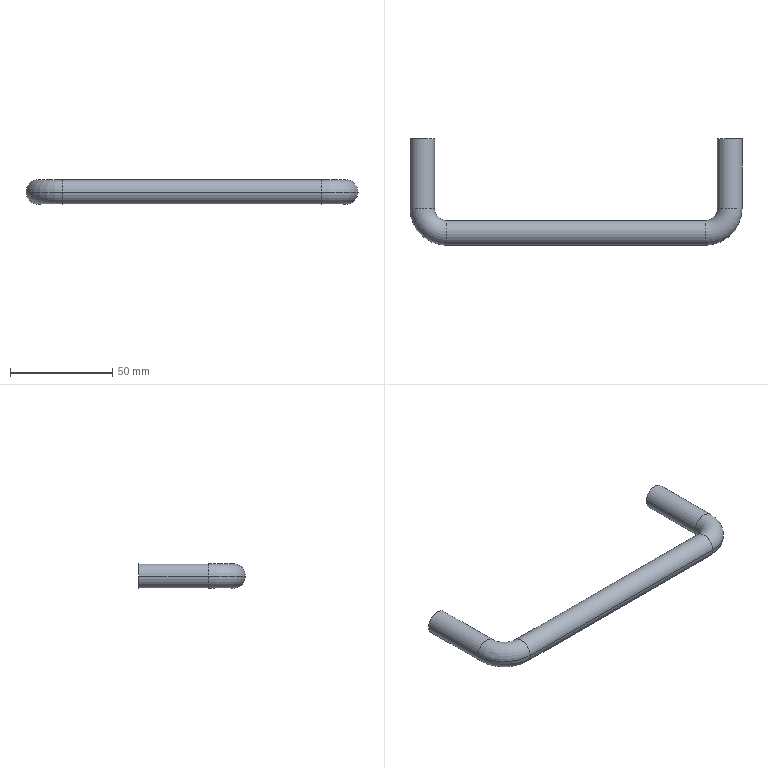Part | NX | 1 solid | 28 faces | box 162 x 52 x 12 mm | volume 24430 mm3 | cylinder 14 | cone 8 | torus 4 | plane 2 | commonest cylinder face diameters 6.8 x8 12 x6
STEP:
#1=CARTESIAN_POINT('',(-81.,0.,0.));
#2=VERTEX_POINT('',#1);
#3=CARTESIAN_POINT('',(-69.,0.,0.));
#4=VERTEX_POINT('',#3);
#5=CARTESIAN_POINT('',(-75.,0.,0.));
#6=DIRECTION('',(0.,-1.,0.));
#7=DIRECTION('',(1.,0.,0.));
#8=AXIS2_PLACEMENT_3D('',#5,#6,#7);
#9=CIRCLE('',#8,6.);
#10=EDGE_CURVE('',#2,#4,#9,.T.);
#11=ORIENTED_EDGE('',*,*,#10,.F.);
#12=CARTESIAN_POINT('',(-75.,0.,0.));
#13=DIRECTION('',(0.,-1.,0.));
#14=DIRECTION('',(1.,0.,0.));
#15=AXIS2_PLACEMENT_3D('',#12,#13,#14);
#16=CIRCLE('',#15,6.);
#17=EDGE_CURVE('',#4,#2,#16,.T.);
#18=ORIENTED_EDGE('',*,*,#17,.F.);
#19=EDGE_LOOP('',(#11,#18));
#20=FACE_BOUND('',#19,.T.);
#21=CARTESIAN_POINT('',(-79.562,0.,0.));
#22=VERTEX_POINT('',#21);
#23=CARTESIAN_POINT('',(-70.438,0.,0.));
#24=VERTEX_POINT('',#23);
#25=CARTESIAN_POINT('',(-75.,0.,0.));
#26=DIRECTION('',(0.,1.,0.));
#27=DIRECTION('',(1.,0.,0.));
#28=AXIS2_PLACEMENT_3D('',#25,#26,#27);
#29=CIRCLE('',#28,4.562);
#30=EDGE_CURVE('',#22,#24,#29,.T.);
#31=ORIENTED_EDGE('',*,*,#30,.F.);
#32=CARTESIAN_POINT('',(-75.,0.,0.));
#33=DIRECTION('',(0.,1.,0.));
#34=DIRECTION('',(1.,0.,0.));
#35=AXIS2_PLACEMENT_3D('',#32,#33,#34);
#36=CIRCLE('',#35,4.562);
#37=EDGE_CURVE('',#24,#22,#36,.T.);
#38=ORIENTED_EDGE('',*,*,#37,.F.);
#39=EDGE_LOOP('',(#31,#38));
#40=FACE_BOUND('',#39,.T.);
#41=CARTESIAN_POINT('',(-75.,0.,0.));
#42=DIRECTION('',(0.,-1.,0.));
#43=DIRECTION('',(0.,0.,-1.));
#44=AXIS2_PLACEMENT_3D('',#41,#42,#43);
#45=PLANE('',#44);
#46=ADVANCED_FACE('',(#20,#40),#45,.F.);
#47=CARTESIAN_POINT('',(-81.,-34.,0.));
#48=VERTEX_POINT('',#47);
#49=CARTESIAN_POINT('',(-69.,-34.,0.));
#50=VERTEX_POINT('',#49);
#51=CARTESIAN_POINT('',(-75.,-34.,0.));
#52=DIRECTION('',(0.,1.,0.));
#53=DIRECTION('',(1.,0.,0.));
#54=AXIS2_PLACEMENT_3D('',#51,#52,#53);
#55=CIRCLE('',#54,6.);
#56=EDGE_CURVE('',#48,#50,#55,.T.);
#57=ORIENTED_EDGE('',*,*,#56,.T.);
#58=CARTESIAN_POINT('',(-69.,0.,0.));
#59=DIRECTION('',(0.,-1.,0.));
#60=VECTOR('',#59,1000.);
#61=LINE('',#58,#60);
#62=EDGE_CURVE('',#4,#50,#61,.T.);
#63=ORIENTED_EDGE('',*,*,#62,.F.);
#64=ORIENTED_EDGE('',*,*,#17,.T.);
#65=CARTESIAN_POINT('',(-81.,0.,0.));
#66=DIRECTION('',(0.,-1.,0.));
#67=VECTOR('',#66,1000.);
#68=LINE('',#65,#67);
#69=EDGE_CURVE('',#2,#48,#68,.T.);
#70=ORIENTED_EDGE('',*,*,#69,.T.);
#71=EDGE_LOOP('',(#57,#63,#64,#70));
#72=FACE_BOUND('',#71,.T.);
#73=CARTESIAN_POINT('',(-75.,0.,0.));
#74=DIRECTION('',(0.,-1.,0.));
#75=DIRECTION('',(1.,0.,0.));
#76=AXIS2_PLACEMENT_3D('',#73,#74,#75);
#77=CYLINDRICAL_SURFACE('',#76,6.);
#78=ADVANCED_FACE('',(#72),#77,.T.);
#79=CARTESIAN_POINT('',(81.,0.,0.));
#80=VERTEX_POINT('',#79);
#81=CARTESIAN_POINT('',(69.,0.,0.));
#82=VERTEX_POINT('',#81);
#83=CARTESIAN_POINT('',(75.,0.,0.));
#84=DIRECTION('',(0.,1.,0.));
#85=DIRECTION('',(-1.,0.,0.));
#86=AXIS2_PLACEMENT_3D('',#83,#84,#85);
#87=CIRCLE('',#86,6.);
#88=EDGE_CURVE('',#80,#82,#87,.T.);
#89=ORIENTED_EDGE('',*,*,#88,.F.);
#90=CARTESIAN_POINT('',(81.,-34.,0.));
#91=VERTEX_POINT('',#90);
#92=CARTESIAN_POINT('',(81.,-34.,0.));
#93=DIRECTION('',(0.,1.,0.));
#94=VECTOR('',#93,1000.);
#95=LINE('',#92,#94);
#96=EDGE_CURVE('',#80,#91,#95,.F.);
#97=ORIENTED_EDGE('',*,*,#96,.T.);
#98=CARTESIAN_POINT('',(69.,-34.,0.));
#99=VERTEX_POINT('',#98);
#100=CARTESIAN_POINT('',(75.,-34.,0.));
#101=DIRECTION('',(0.,1.,0.));
#102=DIRECTION('',(1.,0.,0.));
#103=AXIS2_PLACEMENT_3D('',#100,#101,#102);
#104=CIRCLE('',#103,6.);
#105=EDGE_CURVE('',#91,#99,#104,.T.);
#106=ORIENTED_EDGE('',*,*,#105,.T.);
#107=CARTESIAN_POINT('',(69.,-34.,0.));
#108=DIRECTION('',(0.,1.,0.));
#109=VECTOR('',#108,1000.);
#110=LINE('',#107,#109);
#111=EDGE_CURVE('',#82,#99,#110,.F.);
#112=ORIENTED_EDGE('',*,*,#111,.F.);
#113=EDGE_LOOP('',(#89,#97,#106,#112));
#114=FACE_BOUND('',#113,.T.);
#115=CARTESIAN_POINT('',(75.,-34.,0.));
#116=DIRECTION('',(0.,1.,0.));
#117=DIRECTION('',(-1.,0.,0.));
#118=AXIS2_PLACEMENT_3D('',#115,#116,#117);
#119=CYLINDRICAL_SURFACE('',#118,6.);
#120=ADVANCED_FACE('',(#114),#119,.T.);
#121=ORIENTED_EDGE('',*,*,#56,.F.);
#122=CARTESIAN_POINT('',(-63.,-52.,0.));
#123=VERTEX_POINT('',#122);
#124=CARTESIAN_POINT('',(-63.,-34.,0.));
#125=DIRECTION('',(0.,0.,1.));
#126=DIRECTION('',(1.,0.,0.));
#127=AXIS2_PLACEMENT_3D('',#124,#125,#126);
#128=CIRCLE('',#127,18.);
#129=EDGE_CURVE('',#123,#48,#128,.F.);
#130=ORIENTED_EDGE('',*,*,#129,.F.);
#131=CARTESIAN_POINT('',(-63.,-40.,0.));
#132=VERTEX_POINT('',#131);
#133=CARTESIAN_POINT('',(-63.,-46.,0.));
#134=DIRECTION('',(1.,0.,0.));
#135=DIRECTION('',(0.,-1.,0.));
#136=AXIS2_PLACEMENT_3D('',#133,#134,#135);
#137=CIRCLE('',#136,6.);
#138=EDGE_CURVE('',#132,#123,#137,.T.);
#139=ORIENTED_EDGE('',*,*,#138,.F.);
#140=CARTESIAN_POINT('',(-63.,-34.,0.));
#141=DIRECTION('',(0.,0.,1.));
#142=DIRECTION('',(1.,0.,0.));
#143=AXIS2_PLACEMENT_3D('',#140,#141,#142);
#144=CIRCLE('',#143,6.);
#145=EDGE_CURVE('',#132,#50,#144,.F.);
#146=ORIENTED_EDGE('',*,*,#145,.T.);
#147=EDGE_LOOP('',(#121,#130,#139,#146));
#148=FACE_BOUND('',#147,.T.);
#149=CARTESIAN_POINT('',(-63.,-34.,0.));
#150=DIRECTION('',(0.,0.,1.));
#151=DIRECTION('',(1.,0.,0.));
#152=AXIS2_PLACEMENT_3D('',#149,#150,#151);
#153=TOROIDAL_SURFACE('',#152,12.,6.);
#154=ADVANCED_FACE('',(#148),#153,.T.);
#155=ORIENTED_EDGE('',*,*,#88,.T.);
#156=CARTESIAN_POINT('',(75.,0.,0.));
#157=DIRECTION('',(0.,1.,0.));
#158=DIRECTION('',(-1.,0.,0.));
#159=AXIS2_PLACEMENT_3D('',#156,#157,#158);
#160=CIRCLE('',#159,6.);
#161=EDGE_CURVE('',#82,#80,#160,.T.);
#162=ORIENTED_EDGE('',*,*,#161,.T.);
#163=EDGE_LOOP('',(#155,#162));
#164=FACE_BOUND('',#163,.T.);
#165=CARTESIAN_POINT('',(70.438,0.,0.));
#166=VERTEX_POINT('',#165);
#167=CARTESIAN_POINT('',(79.562,0.,0.));
#168=VERTEX_POINT('',#167);
#169=CARTESIAN_POINT('',(75.,0.,0.));
#170=DIRECTION('',(0.,1.,0.));
#171=DIRECTION('',(1.,0.,0.));
#172=AXIS2_PLACEMENT_3D('',#169,#170,#171);
#173=CIRCLE('',#172,4.562);
#174=EDGE_CURVE('',#166,#168,#173,.T.);
#175=ORIENTED_EDGE('',*,*,#174,.F.);
#176=CARTESIAN_POINT('',(75.,0.,0.));
#177=DIRECTION('',(0.,1.,0.));
#178=DIRECTION('',(1.,0.,0.));
#179=AXIS2_PLACEMENT_3D('',#176,#177,#178);
#180=CIRCLE('',#179,4.562);
#181=EDGE_CURVE('',#168,#166,#180,.T.);
#182=ORIENTED_EDGE('',*,*,#181,.F.);
#183=EDGE_LOOP('',(#175,#182));
#184=FACE_BOUND('',#183,.T.);
#185=CARTESIAN_POINT('',(75.,0.,0.));
#186=DIRECTION('',(0.,1.,0.));
#187=DIRECTION('',(1.,0.,0.));
#188=AXIS2_PLACEMENT_3D('',#185,#186,#187);
#189=PLANE('',#188);
#190=ADVANCED_FACE('',(#164,#184),#189,.T.);
#191=CARTESIAN_POINT('',(-63.,-46.,0.));
#192=DIRECTION('',(1.,0.,0.));
#193=DIRECTION('',(0.,-1.,0.));
#194=AXIS2_PLACEMENT_3D('',#191,#192,#193);
#195=CIRCLE('',#194,6.);
#196=EDGE_CURVE('',#123,#132,#195,.T.);
#197=ORIENTED_EDGE('',*,*,#196,.T.);
#198=CARTESIAN_POINT('',(63.,-40.,0.));
#199=VERTEX_POINT('',#198);
#200=CARTESIAN_POINT('',(-63.,-40.,0.));
#201=DIRECTION('',(1.,0.,0.));
#202=VECTOR('',#201,1000.);
#203=LINE('',#200,#202);
#204=EDGE_CURVE('',#132,#199,#203,.T.);
#205=ORIENTED_EDGE('',*,*,#204,.T.);
#206=CARTESIAN_POINT('',(63.,-52.,0.));
#207=VERTEX_POINT('',#206);
#208=CARTESIAN_POINT('',(63.,-46.,0.));
#209=DIRECTION('',(-1.,0.,0.));
#210=DIRECTION('',(0.,1.,0.));
#211=AXIS2_PLACEMENT_3D('',#208,#209,#210);
#212=CIRCLE('',#211,6.);
#213=EDGE_CURVE('',#199,#207,#212,.T.);
#214=ORIENTED_EDGE('',*,*,#213,.T.);
#215=CARTESIAN_POINT('',(-63.,-52.,0.));
#216=DIRECTION('',(1.,0.,0.));
#217=VECTOR('',#216,1000.);
#218=LINE('',#215,#217);
#219=EDGE_CURVE('',#123,#207,#218,.T.);
#220=ORIENTED_EDGE('',*,*,#219,.F.);
#221=EDGE_LOOP('',(#197,#205,#214,#220));
#222=FACE_BOUND('',#221,.T.);
#223=CARTESIAN_POINT('',(-63.,-46.,0.));
#224=DIRECTION('',(1.,0.,0.));
#225=DIRECTION('',(0.,1.,0.));
#226=AXIS2_PLACEMENT_3D('',#223,#224,#225);
#227=CYLINDRICAL_SURFACE('',#226,6.);
#228=ADVANCED_FACE('',(#222),#227,.T.);
#229=ORIENTED_EDGE('',*,*,#105,.F.);
#230=CARTESIAN_POINT('',(63.,-34.,0.));
#231=DIRECTION('',(0.,0.,1.));
#232=DIRECTION('',(1.,0.,0.));
#233=AXIS2_PLACEMENT_3D('',#230,#231,#232);
#234=CIRCLE('',#233,18.);
#235=EDGE_CURVE('',#91,#207,#234,.F.);
#236=ORIENTED_EDGE('',*,*,#235,.T.);
#237=ORIENTED_EDGE('',*,*,#213,.F.);
#238=CARTESIAN_POINT('',(63.,-34.,0.));
#239=DIRECTION('',(0.,0.,1.));
#240=DIRECTION('',(1.,0.,0.));
#241=AXIS2_PLACEMENT_3D('',#238,#239,#240);
#242=CIRCLE('',#241,6.);
#243=EDGE_CURVE('',#99,#199,#242,.F.);
#244=ORIENTED_EDGE('',*,*,#243,.F.);
#245=EDGE_LOOP('',(#229,#236,#237,#244));
#246=FACE_BOUND('',#245,.T.);
#247=CARTESIAN_POINT('',(63.,-34.,0.));
#248=DIRECTION('',(0.,0.,1.));
#249=DIRECTION('',(1.,0.,0.));
#250=AXIS2_PLACEMENT_3D('',#247,#248,#249);
#251=TOROIDAL_SURFACE('',#250,12.,6.);
#252=ADVANCED_FACE('',(#246),#251,.T.);
#253=CARTESIAN_POINT('',(71.6,-0.6712,0.));
#254=VERTEX_POINT('',#253);
#255=CARTESIAN_POINT('',(78.4,-0.6712,0.));
#256=VERTEX_POINT('',#255);
#257=CARTESIAN_POINT('',(75.,-0.6712,0.));
#258=DIRECTION('',(0.,1.,0.));
#259=DIRECTION('',(1.,0.,0.));
#260=AXIS2_PLACEMENT_3D('',#257,#258,#259);
#261=CIRCLE('',#260,3.4);
#262=EDGE_CURVE('',#254,#256,#261,.T.);
#263=ORIENTED_EDGE('',*,*,#262,.T.);
#264=CARTESIAN_POINT('',(78.4,-16.,0.));
#265=VERTEX_POINT('',#264);
#266=CARTESIAN_POINT('',(78.4,0.,0.));
#267=DIRECTION('',(0.,1.,0.));
#268=VECTOR('',#267,1000.);
#269=LINE('',#266,#268);
#270=EDGE_CURVE('',#265,#256,#269,.T.);
#271=ORIENTED_EDGE('',*,*,#270,.F.);
#272=CARTESIAN_POINT('',(71.6,-16.,0.));
#273=VERTEX_POINT('',#272);
#274=CARTESIAN_POINT('',(75.,-16.,0.));
#275=DIRECTION('',(0.,1.,0.));
#276=DIRECTION('',(1.,0.,0.));
#277=AXIS2_PLACEMENT_3D('',#274,#275,#276);
#278=CIRCLE('',#277,3.4);
#279=EDGE_CURVE('',#273,#265,#278,.T.);
#280=ORIENTED_EDGE('',*,*,#279,.F.);
#281=CARTESIAN_POINT('',(71.6,0.,0.));
#282=DIRECTION('',(0.,1.,0.));
#283=VECTOR('',#282,1000.);
#284=LINE('',#281,#283);
#285=EDGE_CURVE('',#273,#254,#284,.T.);
#286=ORIENTED_EDGE('',*,*,#285,.T.);
#287=EDGE_LOOP('',(#263,#271,#280,#286));
#288=FACE_BOUND('',#287,.T.);
#289=CARTESIAN_POINT('',(75.,0.,0.));
#290=DIRECTION('',(0.,1.,0.));
#291=DIRECTION('',(1.,0.,0.));
#292=AXIS2_PLACEMENT_3D('',#289,#290,#291);
#293=CYLINDRICAL_SURFACE('',#292,3.4);
#294=ADVANCED_FACE('',(#288),#293,.F.);
#295=ORIENTED_EDGE('',*,*,#279,.T.);
#296=CARTESIAN_POINT('',(78.4,-23.5,0.));
#297=VERTEX_POINT('',#296);
#298=CARTESIAN_POINT('',(78.4,0.,0.));
#299=DIRECTION('',(0.,1.,0.));
#300=VECTOR('',#299,1000.);
#301=LINE('',#298,#300);
#302=EDGE_CURVE('',#297,#265,#301,.T.);
#303=ORIENTED_EDGE('',*,*,#302,.F.);
#304=CARTESIAN_POINT('',(71.6,-23.5,0.));
#305=VERTEX_POINT('',#304);
#306=CARTESIAN_POINT('',(75.,-23.5,0.));
#307=DIRECTION('',(0.,1.,0.));
#308=DIRECTION('',(1.,0.,0.));
#309=AXIS2_PLACEMENT_3D('',#306,#307,#308);
#310=CIRCLE('',#309,3.4);
#311=EDGE_CURVE('',#305,#297,#310,.T.);
#312=ORIENTED_EDGE('',*,*,#311,.F.);
#313=CARTESIAN_POINT('',(71.6,0.,0.));
#314=DIRECTION('',(0.,1.,0.));
#315=VECTOR('',#314,1000.);
#316=LINE('',#313,#315);
#317=EDGE_CURVE('',#305,#273,#316,.T.);
#318=ORIENTED_EDGE('',*,*,#317,.T.);
#319=EDGE_LOOP('',(#295,#303,#312,#318));
#320=FACE_BOUND('',#319,.T.);
#321=CARTESIAN_POINT('',(75.,0.,0.));
#322=DIRECTION('',(0.,1.,0.));
#323=DIRECTION('',(1.,0.,0.));
#324=AXIS2_PLACEMENT_3D('',#321,#322,#323);
#325=CYLINDRICAL_SURFACE('',#324,3.4);
#326=ADVANCED_FACE('',(#320),#325,.F.);
#327=ORIENTED_EDGE('',*,*,#311,.T.);
#328=CARTESIAN_POINT('',(75.,-25.543,0.));
#329=VERTEX_POINT('',#328);
#330=CARTESIAN_POINT('',(78.4,-23.5,0.));
#331=DIRECTION('',(0.8572,0.515,0.));
#332=VECTOR('',#331,1000.);
#333=LINE('',#330,#332);
#334=EDGE_CURVE('',#297,#329,#333,.F.);
#335=ORIENTED_EDGE('',*,*,#334,.T.);
#336=CARTESIAN_POINT('',(71.6,-23.5,0.));
#337=DIRECTION('',(-0.8572,0.515,0.));
#338=VECTOR('',#337,1000.);
#339=LINE('',#336,#338);
#340=EDGE_CURVE('',#305,#329,#339,.F.);
#341=ORIENTED_EDGE('',*,*,#340,.F.);
#342=EDGE_LOOP('',(#327,#335,#341));
#343=FACE_BOUND('',#342,.T.);
#344=CARTESIAN_POINT('',(75.,-23.5,0.));
#345=DIRECTION('',(0.,1.,0.));
#346=DIRECTION('',(1.,0.,0.));
#347=AXIS2_PLACEMENT_3D('',#344,#345,#346);
#348=CONICAL_SURFACE('',#347,3.4,1.03);
#349=ADVANCED_FACE('',(#343),#348,.F.);
#350=ORIENTED_EDGE('',*,*,#262,.F.);
#351=CARTESIAN_POINT('',(71.6,-0.6712,0.));
#352=DIRECTION('',(-0.866,0.5,0.));
#353=VECTOR('',#352,1000.);
#354=LINE('',#351,#353);
#355=EDGE_CURVE('',#254,#166,#354,.T.);
#356=ORIENTED_EDGE('',*,*,#355,.T.);
#357=ORIENTED_EDGE('',*,*,#174,.T.);
#358=CARTESIAN_POINT('',(78.4,-0.6712,0.));
#359=DIRECTION('',(0.866,0.5,0.));
#360=VECTOR('',#359,1000.);
#361=LINE('',#358,#360);
#362=EDGE_CURVE('',#256,#168,#361,.T.);
#363=ORIENTED_EDGE('',*,*,#362,.F.);
#364=EDGE_LOOP('',(#350,#356,#357,#363));
#365=FACE_BOUND('',#364,.T.);
#366=CARTESIAN_POINT('',(75.,-0.6712,0.));
#367=DIRECTION('',(0.,1.,0.));
#368=DIRECTION('',(1.,0.,0.));
#369=AXIS2_PLACEMENT_3D('',#366,#367,#368);
#370=CONICAL_SURFACE('',#369,3.4,1.047);
#371=ADVANCED_FACE('',(#365),#370,.F.);
#372=CARTESIAN_POINT('',(-78.4,-0.6712,0.));
#373=VERTEX_POINT('',#372);
#374=CARTESIAN_POINT('',(-71.6,-0.6712,0.));
#375=VERTEX_POINT('',#374);
#376=CARTESIAN_POINT('',(-75.,-0.6712,0.));
#377=DIRECTION('',(0.,1.,0.));
#378=DIRECTION('',(1.,0.,0.));
#379=AXIS2_PLACEMENT_3D('',#376,#377,#378);
#380=CIRCLE('',#379,3.4);
#381=EDGE_CURVE('',#373,#375,#380,.T.);
#382=ORIENTED_EDGE('',*,*,#381,.T.);
#383=CARTESIAN_POINT('',(-71.6,-16.,0.));
#384=VERTEX_POINT('',#383);
#385=CARTESIAN_POINT('',(-71.6,0.,0.));
#386=DIRECTION('',(0.,1.,0.));
#387=VECTOR('',#386,1000.);
#388=LINE('',#385,#387);
#389=EDGE_CURVE('',#384,#375,#388,.T.);
#390=ORIENTED_EDGE('',*,*,#389,.F.);
#391=CARTESIAN_POINT('',(-78.4,-16.,0.));
#392=VERTEX_POINT('',#391);
#393=CARTESIAN_POINT('',(-75.,-16.,0.));
#394=DIRECTION('',(0.,1.,0.));
#395=DIRECTION('',(1.,0.,0.));
#396=AXIS2_PLACEMENT_3D('',#393,#394,#395);
#397=CIRCLE('',#396,3.4);
#398=EDGE_CURVE('',#392,#384,#397,.T.);
#399=ORIENTED_EDGE('',*,*,#398,.F.);
#400=CARTESIAN_POINT('',(-78.4,0.,0.));
#401=DIRECTION('',(0.,1.,0.));
#402=VECTOR('',#401,1000.);
#403=LINE('',#400,#402);
#404=EDGE_CURVE('',#392,#373,#403,.T.);
#405=ORIENTED_EDGE('',*,*,#404,.T.);
#406=EDGE_LOOP('',(#382,#390,#399,#405));
#407=FACE_BOUND('',#406,.T.);
#408=CARTESIAN_POINT('',(-75.,0.,0.));
#409=DIRECTION('',(0.,1.,0.));
#410=DIRECTION('',(1.,0.,0.));
#411=AXIS2_PLACEMENT_3D('',#408,#409,#410);
#412=CYLINDRICAL_SURFACE('',#411,3.4);
#413=ADVANCED_FACE('',(#407),#412,.F.);
#414=ORIENTED_EDGE('',*,*,#398,.T.);
#415=CARTESIAN_POINT('',(-71.6,-23.5,0.));
#416=VERTEX_POINT('',#415);
#417=CARTESIAN_POINT('',(-71.6,0.,0.));
#418=DIRECTION('',(0.,1.,0.));
#419=VECTOR('',#418,1000.);
#420=LINE('',#417,#419);
#421=EDGE_CURVE('',#416,#384,#420,.T.);
#422=ORIENTED_EDGE('',*,*,#421,.F.);
#423=CARTESIAN_POINT('',(-78.4,-23.5,0.));
#424=VERTEX_POINT('',#423);
#425=CARTESIAN_POINT('',(-75.,-23.5,0.));
#426=DIRECTION('',(0.,1.,0.));
#427=DIRECTION('',(1.,0.,0.));
#428=AXIS2_PLACEMENT_3D('',#425,#426,#427);
#429=CIRCLE('',#428,3.4);
#430=EDGE_CURVE('',#424,#416,#429,.T.);
#431=ORIENTED_EDGE('',*,*,#430,.F.);
#432=CARTESIAN_POINT('',(-78.4,0.,0.));
#433=DIRECTION('',(0.,1.,0.));
#434=VECTOR('',#433,1000.);
#435=LINE('',#432,#434);
#436=EDGE_CURVE('',#424,#392,#435,.T.);
#437=ORIENTED_EDGE('',*,*,#436,.T.);
#438=EDGE_LOOP('',(#414,#422,#431,#437));
#439=FACE_BOUND('',#438,.T.);
#440=CARTESIAN_POINT('',(-75.,0.,0.));
#441=DIRECTION('',(0.,1.,0.));
#442=DIRECTION('',(1.,0.,0.));
#443=AXIS2_PLACEMENT_3D('',#440,#441,#442);
#444=CYLINDRICAL_SURFACE('',#443,3.4);
#445=ADVANCED_FACE('',(#439),#444,.F.);
#446=ORIENTED_EDGE('',*,*,#430,.T.);
#447=CARTESIAN_POINT('',(-75.,-25.543,0.));
#448=VERTEX_POINT('',#447);
#449=CARTESIAN_POINT('',(-71.6,-23.5,0.));
#450=DIRECTION('',(0.8572,0.515,0.));
#451=VECTOR('',#450,1000.);
#452=LINE('',#449,#451);
#453=EDGE_CURVE('',#416,#448,#452,.F.);
#454=ORIENTED_EDGE('',*,*,#453,.T.);
#455=CARTESIAN_POINT('',(-78.4,-23.5,0.));
#456=DIRECTION('',(-0.8572,0.515,0.));
#457=VECTOR('',#456,1000.);
#458=LINE('',#455,#457);
#459=EDGE_CURVE('',#424,#448,#458,.F.);
#460=ORIENTED_EDGE('',*,*,#459,.F.);
#461=EDGE_LOOP('',(#446,#454,#460));
#462=FACE_BOUND('',#461,.T.);
#463=CARTESIAN_POINT('',(-75.,-23.5,0.));
#464=DIRECTION('',(0.,1.,0.));
#465=DIRECTION('',(1.,0.,0.));
#466=AXIS2_PLACEMENT_3D('',#463,#464,#465);
#467=CONICAL_SURFACE('',#466,3.4,1.03);
#468=ADVANCED_FACE('',(#462),#467,.F.);
#469=ORIENTED_EDGE('',*,*,#381,.F.);
#470=CARTESIAN_POINT('',(-78.4,-0.6712,0.));
#471=DIRECTION('',(-0.866,0.5,0.));
#472=VECTOR('',#471,1000.);
#473=LINE('',#470,#472);
#474=EDGE_CURVE('',#373,#22,#473,.T.);
#475=ORIENTED_EDGE('',*,*,#474,.T.);
#476=ORIENTED_EDGE('',*,*,#30,.T.);
#477=CARTESIAN_POINT('',(-71.6,-0.6712,0.));
#478=DIRECTION('',(0.866,0.5,0.));
#479=VECTOR('',#478,1000.);
#480=LINE('',#477,#479);
#481=EDGE_CURVE('',#375,#24,#480,.T.);
#482=ORIENTED_EDGE('',*,*,#481,.F.);
#483=EDGE_LOOP('',(#469,#475,#476,#482));
#484=FACE_BOUND('',#483,.T.);
#485=CARTESIAN_POINT('',(-75.,-0.6712,0.));
#486=DIRECTION('',(0.,1.,0.));
#487=DIRECTION('',(1.,0.,0.));
#488=AXIS2_PLACEMENT_3D('',#485,#486,#487);
#489=CONICAL_SURFACE('',#488,3.4,1.047);
#490=ADVANCED_FACE('',(#484),#489,.F.);
#491=ORIENTED_EDGE('',*,*,#340,.T.);
#492=ORIENTED_EDGE('',*,*,#334,.F.);
#493=CARTESIAN_POINT('',(75.,-23.5,0.));
#494=DIRECTION('',(0.,1.,0.));
#495=DIRECTION('',(1.,0.,0.));
#496=AXIS2_PLACEMENT_3D('',#493,#494,#495);
#497=CIRCLE('',#496,3.4);
#498=EDGE_CURVE('',#297,#305,#497,.T.);
#499=ORIENTED_EDGE('',*,*,#498,.T.);
#500=EDGE_LOOP('',(#491,#492,#499));
#501=FACE_BOUND('',#500,.T.);
#502=CARTESIAN_POINT('',(75.,-23.5,0.));
#503=DIRECTION('',(0.,1.,0.));
#504=DIRECTION('',(1.,0.,0.));
#505=AXIS2_PLACEMENT_3D('',#502,#503,#504);
#506=CONICAL_SURFACE('',#505,3.4,1.03);
#507=ADVANCED_FACE('',(#501),#506,.F.);
#508=ORIENTED_EDGE('',*,*,#362,.T.);
#509=ORIENTED_EDGE('',*,*,#181,.T.);
#510=ORIENTED_EDGE('',*,*,#355,.F.);
#511=CARTESIAN_POINT('',(75.,-0.6712,0.));
#512=DIRECTION('',(0.,1.,0.));
#513=DIRECTION('',(1.,0.,0.));
#514=AXIS2_PLACEMENT_3D('',#511,#512,#513);
#515=CIRCLE('',#514,3.4);
#516=EDGE_CURVE('',#256,#254,#515,.T.);
#517=ORIENTED_EDGE('',*,*,#516,.F.);
#518=EDGE_LOOP('',(#508,#509,#510,#517));
#519=FACE_BOUND('',#518,.T.);
#520=CARTESIAN_POINT('',(75.,-0.6712,0.));
#521=DIRECTION('',(0.,1.,0.));
#522=DIRECTION('',(1.,0.,0.));
#523=AXIS2_PLACEMENT_3D('',#520,#521,#522);
#524=CONICAL_SURFACE('',#523,3.4,1.047);
#525=ADVANCED_FACE('',(#519),#524,.F.);
#526=ORIENTED_EDGE('',*,*,#111,.T.);
#527=CARTESIAN_POINT('',(75.,-34.,0.));
#528=DIRECTION('',(0.,1.,0.));
#529=DIRECTION('',(1.,0.,0.));
#530=AXIS2_PLACEMENT_3D('',#527,#528,#529);
#531=CIRCLE('',#530,6.);
#532=EDGE_CURVE('',#99,#91,#531,.T.);
#533=ORIENTED_EDGE('',*,*,#532,.T.);
#534=ORIENTED_EDGE('',*,*,#96,.F.);
#535=ORIENTED_EDGE('',*,*,#161,.F.);
#536=EDGE_LOOP('',(#526,#533,#534,#535));
#537=FACE_BOUND('',#536,.T.);
#538=CARTESIAN_POINT('',(75.,-34.,0.));
#539=DIRECTION('',(0.,1.,0.));
#540=DIRECTION('',(-1.,0.,0.));
#541=AXIS2_PLACEMENT_3D('',#538,#539,#540);
#542=CYLINDRICAL_SURFACE('',#541,6.);
#543=ADVANCED_FACE('',(#537),#542,.T.);
#544=ORIENTED_EDGE('',*,*,#196,.F.);
#545=ORIENTED_EDGE('',*,*,#129,.T.);
#546=CARTESIAN_POINT('',(-75.,-34.,0.));
#547=DIRECTION('',(0.,1.,0.));
#548=DIRECTION('',(1.,0.,0.));
#549=AXIS2_PLACEMENT_3D('',#546,#547,#548);
#550=CIRCLE('',#549,6.);
#551=EDGE_CURVE('',#50,#48,#550,.T.);
#552=ORIENTED_EDGE('',*,*,#551,.F.);
#553=ORIENTED_EDGE('',*,*,#145,.F.);
#554=EDGE_LOOP('',(#544,#545,#552,#553));
#555=FACE_BOUND('',#554,.T.);
#556=CARTESIAN_POINT('',(-63.,-34.,0.));
#557=DIRECTION('',(0.,0.,1.));
#558=DIRECTION('',(1.,0.,0.));
#559=AXIS2_PLACEMENT_3D('',#556,#557,#558);
#560=TOROIDAL_SURFACE('',#559,12.,6.);
#561=ADVANCED_FACE('',(#555),#560,.T.);
#562=ORIENTED_EDGE('',*,*,#421,.T.);
#563=CARTESIAN_POINT('',(-75.,-16.,0.));
#564=DIRECTION('',(0.,1.,0.));
#565=DIRECTION('',(1.,0.,0.));
#566=AXIS2_PLACEMENT_3D('',#563,#564,#565);
#567=CIRCLE('',#566,3.4);
#568=EDGE_CURVE('',#384,#392,#567,.T.);
#569=ORIENTED_EDGE('',*,*,#568,.T.);
#570=ORIENTED_EDGE('',*,*,#436,.F.);
#571=CARTESIAN_POINT('',(-75.,-23.5,0.));
#572=DIRECTION('',(0.,1.,0.));
#573=DIRECTION('',(1.,0.,0.));
#574=AXIS2_PLACEMENT_3D('',#571,#572,#573);
#575=CIRCLE('',#574,3.4);
#576=EDGE_CURVE('',#416,#424,#575,.T.);
#577=ORIENTED_EDGE('',*,*,#576,.F.);
#578=EDGE_LOOP('',(#562,#569,#570,#577));
#579=FACE_BOUND('',#578,.T.);
#580=CARTESIAN_POINT('',(-75.,0.,0.));
#581=DIRECTION('',(0.,1.,0.));
#582=DIRECTION('',(1.,0.,0.));
#583=AXIS2_PLACEMENT_3D('',#580,#581,#582);
#584=CYLINDRICAL_SURFACE('',#583,3.4);
#585=ADVANCED_FACE('',(#579),#584,.F.);
#586=ORIENTED_EDGE('',*,*,#270,.T.);
#587=ORIENTED_EDGE('',*,*,#516,.T.);
#588=ORIENTED_EDGE('',*,*,#285,.F.);
#589=CARTESIAN_POINT('',(75.,-16.,0.));
#590=DIRECTION('',(0.,1.,0.));
#591=DIRECTION('',(1.,0.,0.));
#592=AXIS2_PLACEMENT_3D('',#589,#590,#591);
#593=CIRCLE('',#592,3.4);
#594=EDGE_CURVE('',#265,#273,#593,.T.);
#595=ORIENTED_EDGE('',*,*,#594,.F.);
#596=EDGE_LOOP('',(#586,#587,#588,#595));
#597=FACE_BOUND('',#596,.T.);
#598=CARTESIAN_POINT('',(75.,0.,0.));
#599=DIRECTION('',(0.,1.,0.));
#600=DIRECTION('',(1.,0.,0.));
#601=AXIS2_PLACEMENT_3D('',#598,#599,#600);
#602=CYLINDRICAL_SURFACE('',#601,3.4);
#603=ADVANCED_FACE('',(#597),#602,.F.);
#604=CARTESIAN_POINT('',(63.,-46.,0.));
#605=DIRECTION('',(-1.,0.,0.));
#606=DIRECTION('',(0.,1.,0.));
#607=AXIS2_PLACEMENT_3D('',#604,#605,#606);
#608=CIRCLE('',#607,6.);
#609=EDGE_CURVE('',#207,#199,#608,.T.);
#610=ORIENTED_EDGE('',*,*,#609,.T.);
#611=ORIENTED_EDGE('',*,*,#204,.F.);
#612=ORIENTED_EDGE('',*,*,#138,.T.);
#613=ORIENTED_EDGE('',*,*,#219,.T.);
#614=EDGE_LOOP('',(#610,#611,#612,#613));
#615=FACE_BOUND('',#614,.T.);
#616=CARTESIAN_POINT('',(-63.,-46.,0.));
#617=DIRECTION('',(1.,0.,0.));
#618=DIRECTION('',(0.,1.,0.));
#619=AXIS2_PLACEMENT_3D('',#616,#617,#618);
#620=CYLINDRICAL_SURFACE('',#619,6.);
#621=ADVANCED_FACE('',(#615),#620,.T.);
#622=ORIENTED_EDGE('',*,*,#459,.T.);
#623=ORIENTED_EDGE('',*,*,#453,.F.);
#624=ORIENTED_EDGE('',*,*,#576,.T.);
#625=EDGE_LOOP('',(#622,#623,#624));
#626=FACE_BOUND('',#625,.T.);
#627=CARTESIAN_POINT('',(-75.,-23.5,0.));
#628=DIRECTION('',(0.,1.,0.));
#629=DIRECTION('',(1.,0.,0.));
#630=AXIS2_PLACEMENT_3D('',#627,#628,#629);
#631=CONICAL_SURFACE('',#630,3.4,1.03);
#632=ADVANCED_FACE('',(#626),#631,.F.);
#633=ORIENTED_EDGE('',*,*,#481,.T.);
#634=ORIENTED_EDGE('',*,*,#37,.T.);
#635=ORIENTED_EDGE('',*,*,#474,.F.);
#636=CARTESIAN_POINT('',(-75.,-0.6712,0.));
#637=DIRECTION('',(0.,1.,0.));
#638=DIRECTION('',(1.,0.,0.));
#639=AXIS2_PLACEMENT_3D('',#636,#637,#638);
#640=CIRCLE('',#639,3.4);
#641=EDGE_CURVE('',#375,#373,#640,.T.);
#642=ORIENTED_EDGE('',*,*,#641,.F.);
#643=EDGE_LOOP('',(#633,#634,#635,#642));
#644=FACE_BOUND('',#643,.T.);
#645=CARTESIAN_POINT('',(-75.,-0.6712,0.));
#646=DIRECTION('',(0.,1.,0.));
#647=DIRECTION('',(1.,0.,0.));
#648=AXIS2_PLACEMENT_3D('',#645,#646,#647);
#649=CONICAL_SURFACE('',#648,3.4,1.047);
#650=ADVANCED_FACE('',(#644),#649,.F.);
#651=ORIENTED_EDGE('',*,*,#302,.T.);
#652=ORIENTED_EDGE('',*,*,#594,.T.);
#653=ORIENTED_EDGE('',*,*,#317,.F.);
#654=ORIENTED_EDGE('',*,*,#498,.F.);
#655=EDGE_LOOP('',(#651,#652,#653,#654));
#656=FACE_BOUND('',#655,.T.);
#657=CARTESIAN_POINT('',(75.,0.,0.));
#658=DIRECTION('',(0.,1.,0.));
#659=DIRECTION('',(1.,0.,0.));
#660=AXIS2_PLACEMENT_3D('',#657,#658,#659);
#661=CYLINDRICAL_SURFACE('',#660,3.4);
#662=ADVANCED_FACE('',(#656),#661,.F.);
#663=ORIENTED_EDGE('',*,*,#609,.F.);
#664=ORIENTED_EDGE('',*,*,#235,.F.);
#665=ORIENTED_EDGE('',*,*,#532,.F.);
#666=ORIENTED_EDGE('',*,*,#243,.T.);
#667=EDGE_LOOP('',(#663,#664,#665,#666));
#668=FACE_BOUND('',#667,.T.);
#669=CARTESIAN_POINT('',(63.,-34.,0.));
#670=DIRECTION('',(0.,0.,1.));
#671=DIRECTION('',(1.,0.,0.));
#672=AXIS2_PLACEMENT_3D('',#669,#670,#671);
#673=TOROIDAL_SURFACE('',#672,12.,6.);
#674=ADVANCED_FACE('',(#668),#673,.T.);
#675=ORIENTED_EDGE('',*,*,#10,.T.);
#676=ORIENTED_EDGE('',*,*,#62,.T.);
#677=ORIENTED_EDGE('',*,*,#551,.T.);
#678=ORIENTED_EDGE('',*,*,#69,.F.);
#679=EDGE_LOOP('',(#675,#676,#677,#678));
#680=FACE_BOUND('',#679,.T.);
#681=CARTESIAN_POINT('',(-75.,0.,0.));
#682=DIRECTION('',(0.,-1.,0.));
#683=DIRECTION('',(1.,0.,0.));
#684=AXIS2_PLACEMENT_3D('',#681,#682,#683);
#685=CYLINDRICAL_SURFACE('',#684,6.);
#686=ADVANCED_FACE('',(#680),#685,.T.);
#687=ORIENTED_EDGE('',*,*,#389,.T.);
#688=ORIENTED_EDGE('',*,*,#641,.T.);
#689=ORIENTED_EDGE('',*,*,#404,.F.);
#690=ORIENTED_EDGE('',*,*,#568,.F.);
#691=EDGE_LOOP('',(#687,#688,#689,#690));
#692=FACE_BOUND('',#691,.T.);
#693=CARTESIAN_POINT('',(-75.,0.,0.));
#694=DIRECTION('',(0.,1.,0.));
#695=DIRECTION('',(1.,0.,0.));
#696=AXIS2_PLACEMENT_3D('',#693,#694,#695);
#697=CYLINDRICAL_SURFACE('',#696,3.4);
#698=ADVANCED_FACE('',(#692),#697,.F.);
#699=CLOSED_SHELL('',(#46,#78,#120,#154,#190,#228,#252,#294,#326,#349,#371,#413,#445,#468,#490,#507,#525,#543,#561,#585,#603,#621,#632,#650,#662,#674,#686,#698));
#700=MANIFOLD_SOLID_BREP('',#699);
#701=(LENGTH_UNIT()NAMED_UNIT(*)SI_UNIT(.MILLI.,.METRE.));
#702=UNCERTAINTY_MEASURE_WITH_UNIT(LENGTH_MEASURE(0.00001),#701,'','');
#703=(NAMED_UNIT(*)PLANE_ANGLE_UNIT()SI_UNIT($,.RADIAN.));
#704=(NAMED_UNIT(*)SI_UNIT($,.STERADIAN.)SOLID_ANGLE_UNIT());
#705=(GEOMETRIC_REPRESENTATION_CONTEXT(3)GLOBAL_UNCERTAINTY_ASSIGNED_CONTEXT((#702))GLOBAL_UNIT_ASSIGNED_CONTEXT((#701,#703,#704))REPRESENTATION_CONTEXT('',''));
#706=ADVANCED_BREP_SHAPE_REPRESENTATION('',(#700),#705);